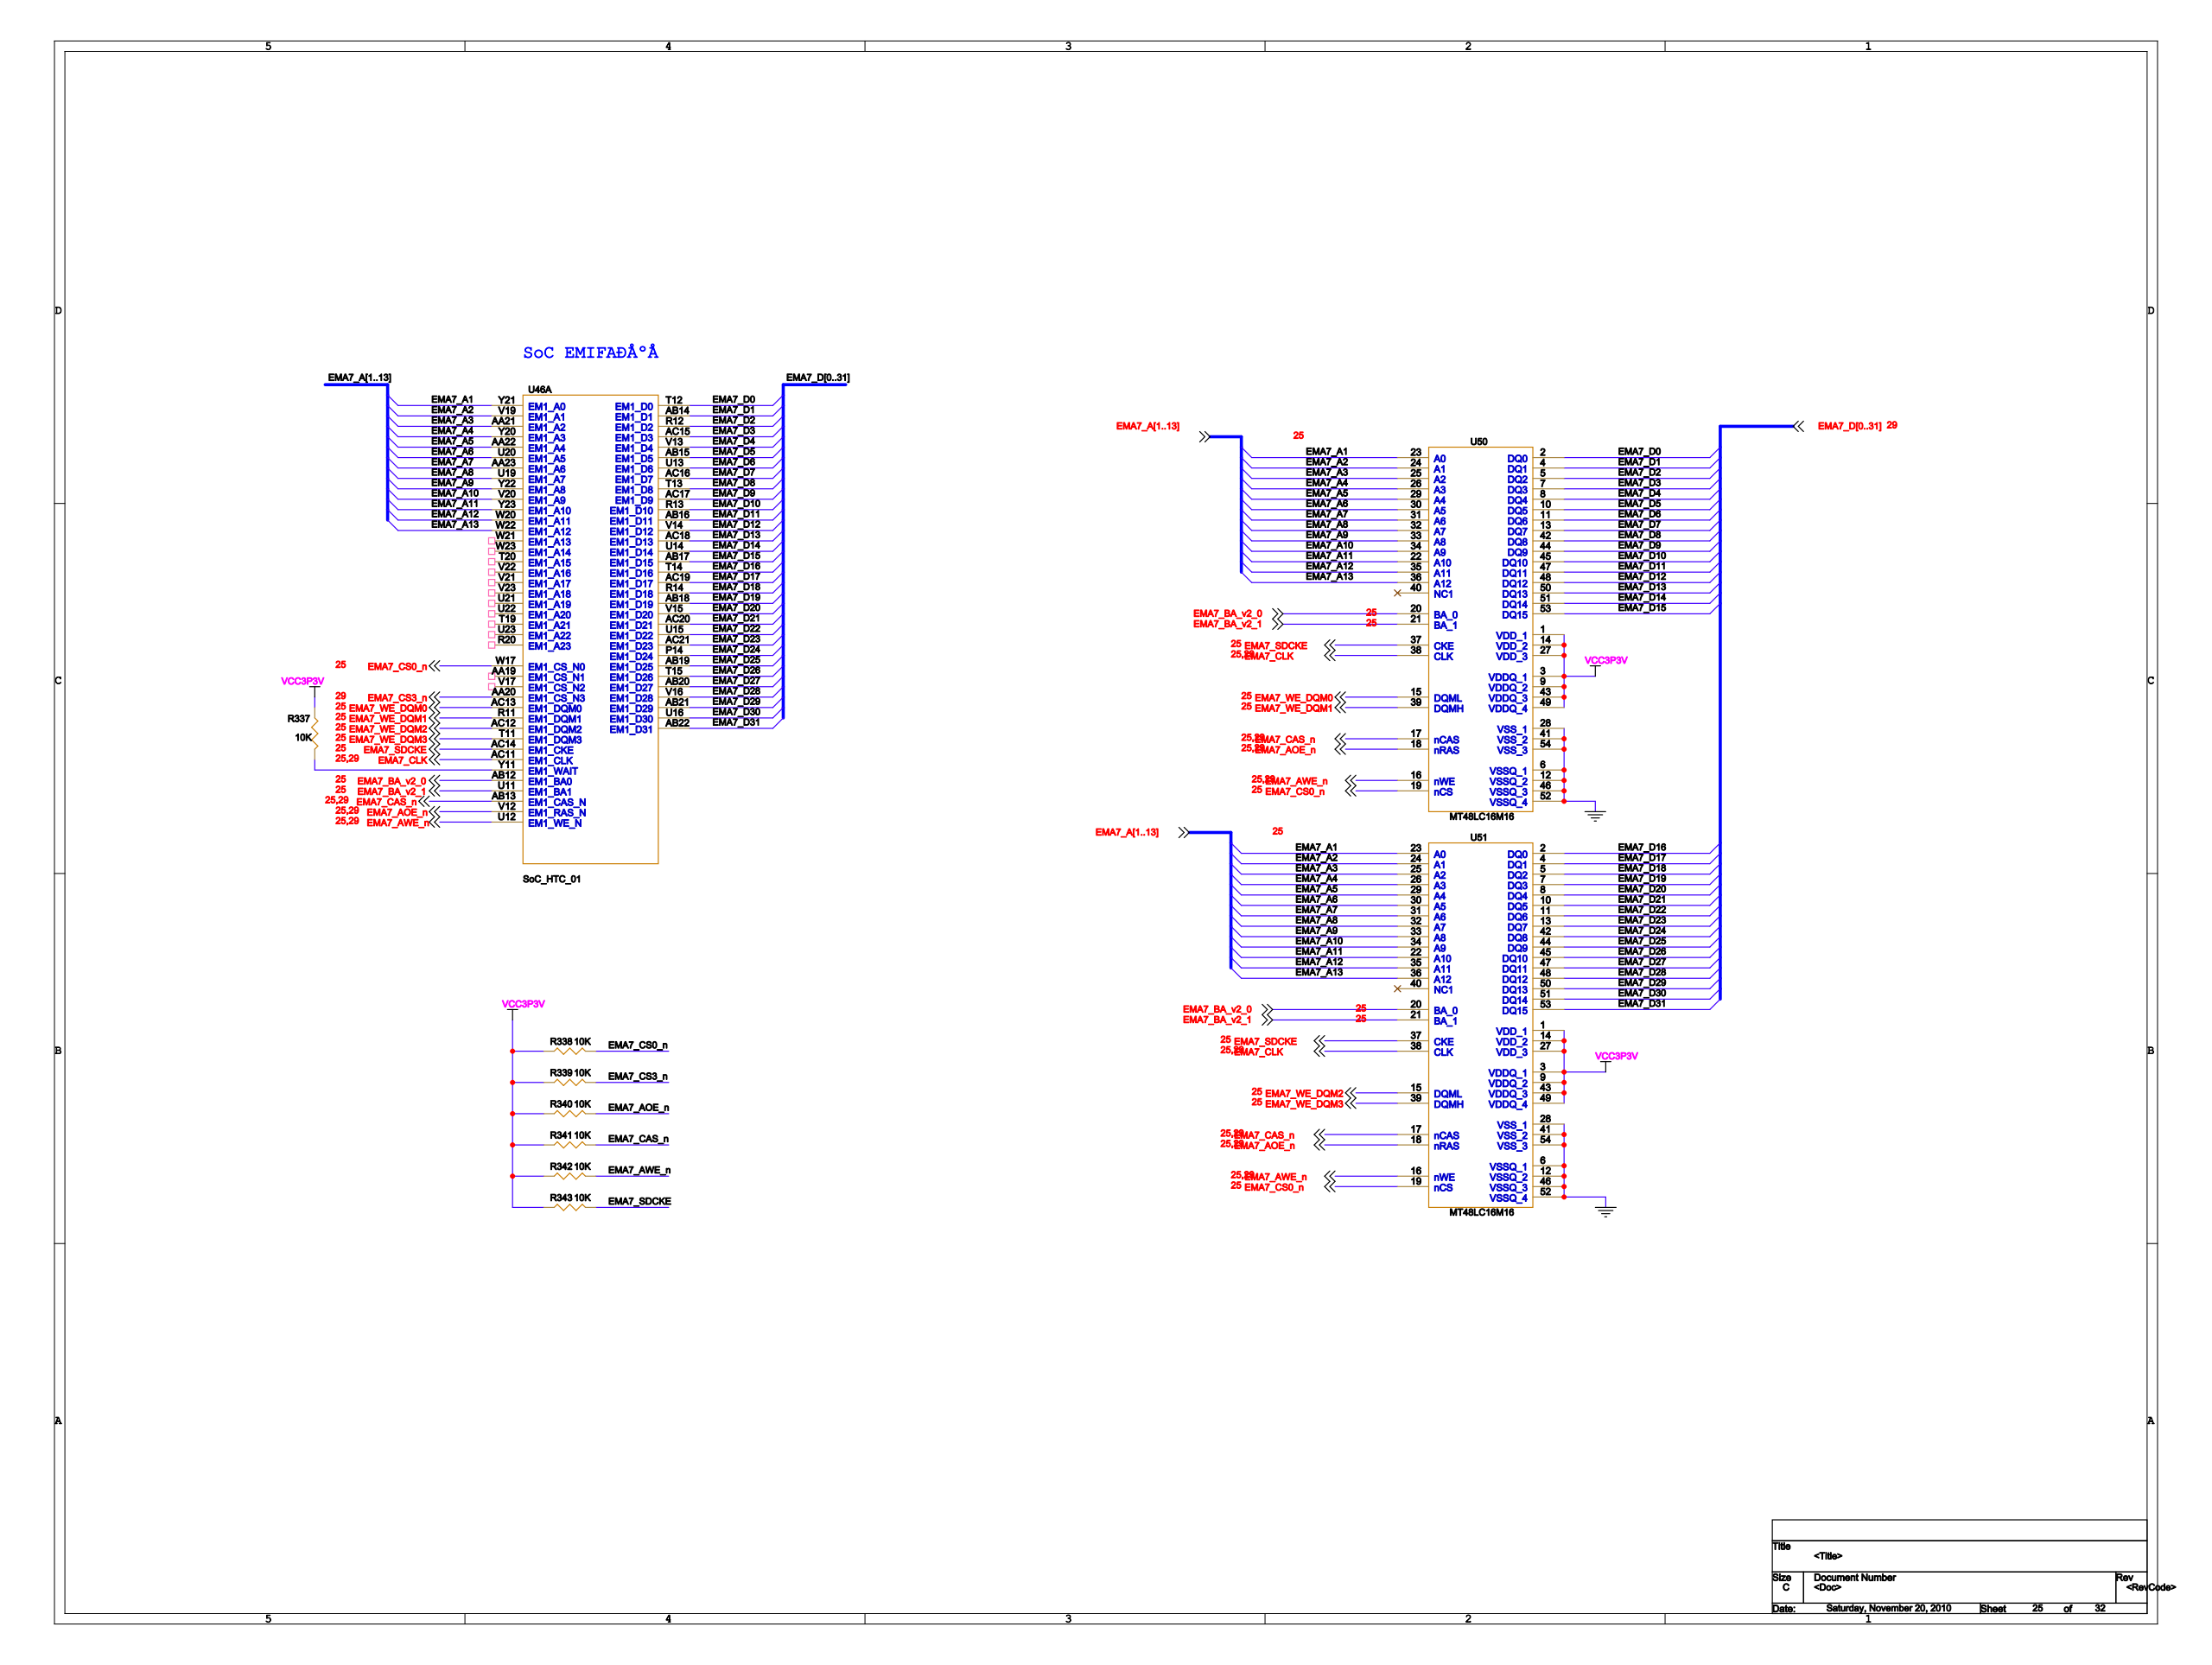Circuit board | Cadence Allegro | 1001 parts | 1318 nets | one sheet of the schematic
Parts on this sheet (reference | value | footprint):
R337 | 10K | 0603
R338 | 10K | 0603
R339 | 10K | 0603
R340 | 10K | 0603
R341 | 10K | 0603
R342 | 10K | 0603
R343 | 10K | 0603
U11 | MT48LC32M16 | TSOP54
U14 | MT48LC16M16 | TSOP54
U15 | MT48LC16M16 | TSOP54
U20 | MT48LC16M16 | TSOP54
U21 | MT48LC16M16 | TSOP54
U23 | MT48LC32M16 | TSOP54
U46 | SoC_HTC_01 | L529_XIN
U50 | MT48LC16M16 | TSOP54
U51 | MT48LC16M16 | TSOP54
Nets of these parts (net: part-pin ...):
EMA7_D28: U46-V16 U51-48
EMA7_D30: U46-U16 U51-51
EMA7_D20: U46-V15 U51-8
EMA7_D24: U46-P14 U51-42
EMA7_D26: U46-T15 U51-45
EMA7_D12: U46-V14 U50-48
EMA7_D22: U46-U15 U51-11
EMA7_D18: U46-R14 U51-5
EMA7_D16: U46-T14 U51-2
EMA7_D19: U46-AB18 U51-7
EMA7_D25: U46-AB19 U51-44
EMA7_D27: U46-AB20 U51-47
EMA7_D9: U46-AC17 U50-44
EMA7_D21: U46-AC20 U51-10
EMA7_D29: U46-AB21 U51-50
EMA7_D23: U46-AC21 U51-13
EMA7_D5: U46-AB15 U50-10
EMA7_D11: U46-AB16 U50-47
EMA7_D15: U46-AB17 U50-53
EMA7_D13: U46-AC18 U50-50
EMA7_CS3_N: R339-2 U46-AA20
EMA7_D31: U46-AB22 U51-53
EMA7_D0: U46-T12 U50-2
EMA7_D2: U46-R12 U50-5
EMA7_D8: U46-T13 U50-42
EMA7_D10: U46-R13 U50-45
EMA7_CLK: U46-AC11 U50-38 U51-38
EMA7_D1: U46-AB14 U50-4
EMA7_D3: U46-AC15 U50-7
EMA7_D17: U46-AC19 U51-4
EMA7_CAS_N: R341-2 U46-AB13 U50-17 U51-17
EMA7_D7: U46-AC16 U50-13
EMA7_D4: U46-V13 U50-8
EMA7_D14: U46-U14 U50-51
EMA7_D6: U46-U13 U50-11
EMA7_AOE_N: R340-2 U46-V12 U50-18 U51-18
EMA7_AWE_N: R342-2 U46-U12 U50-16 U51-16
VCC3P3V: R337-2 R338-1 R339-1 R340-1 R341-1 R342-1 R343-1 U11-1 U11-3 U11-9 U11-14 U11-27 U11-43 U11-49 U14-1 U14-3 U14-9 U14-14 U14-27 U14-43 U14-49 U15-1 U15-3 U15-9 U15-14 U15-27 U15-43 U15-49 U20-1 U20-3 U20-9 U20-14 U20-27 U20-43 U20-49 U21-1 U21-3 U21-9 U21-14 U21-27 U21-43 U21-49 U23-1 U23-3 U23-9 U23-14 U23-27 U23-43 U23-49 U50-1 U50-3 U50-9 U50-14 U50-27 U50-43 U50-49 U51-1 U51-3 U51-9 U51-14 U51-27 U51-43 U51-49
EMA7_A1: U46-Y21 U50-23 U51-23
EMA7_A2: U46-V19 U50-24 U51-24
EMA7_A11: U46-Y23 U50-22 U51-22
EMA7_A12: U46-W20 U50-35 U51-35
EMA7_A13: U46-W22 U50-36 U51-36
EMA7_A3: U46-AA21 U50-25 U51-25
EMA7_A4: U46-Y20 U50-26 U51-26
EMA7_A5: U46-AA22 U50-29 U51-29
EMA7_A6: U46-U20 U50-30 U51-30
EMA7_A7: U46-AA23 U50-31 U51-31
EMA7_A8: U46-U19 U50-32 U51-32
EMA7_A9: U46-Y22 U50-33 U51-33
EMA7_A10: U46-V20 U50-34 U51-34
EMA7_SDCKE: R343-2 U46-AC14 U50-37 U51-37
EMA7_CS0_N: R338-2 U46-W17 U50-19 U51-19
EMA7_WE_DQM0: U46-AC13 U50-15
EMA7_WE_DQM1: U46-R11 U50-39
EMA7_WE_DQM2: U46-AC12 U51-15
EMA7_WE_DQM3: U46-T11 U51-39
N16953386: R337-1 U46-Y11